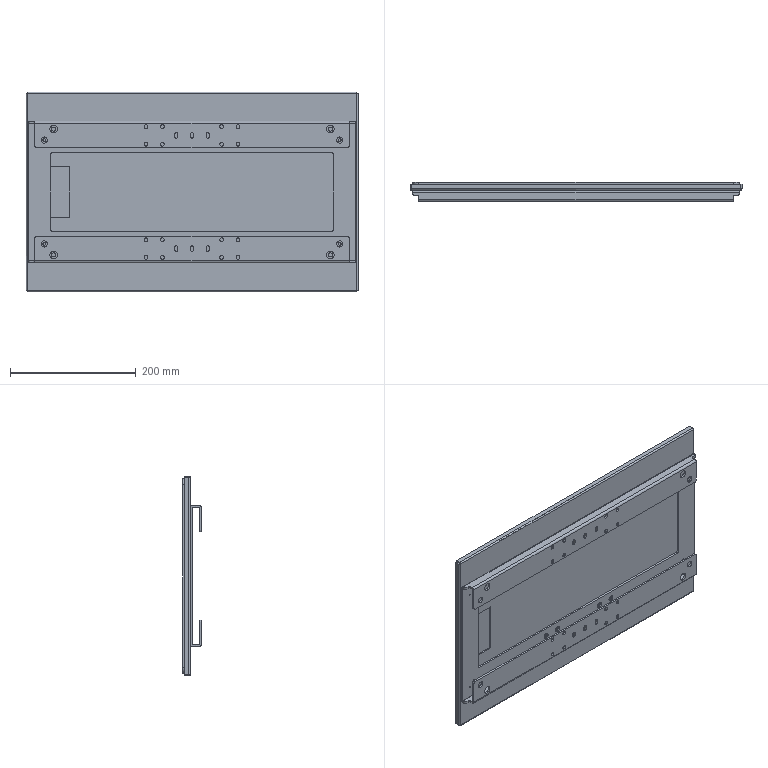Part | SolidWorks | 3 solids | 332 faces | box 528 x 29.8 x 318 mm | volume 2287252 mm3 | cylinder 222 | plane 86 | cone 16 | spline 8 | commonest cylinder face diameters 10 x52 6 x48 9 x44 5 x18 2.5 x16 0.4 x8